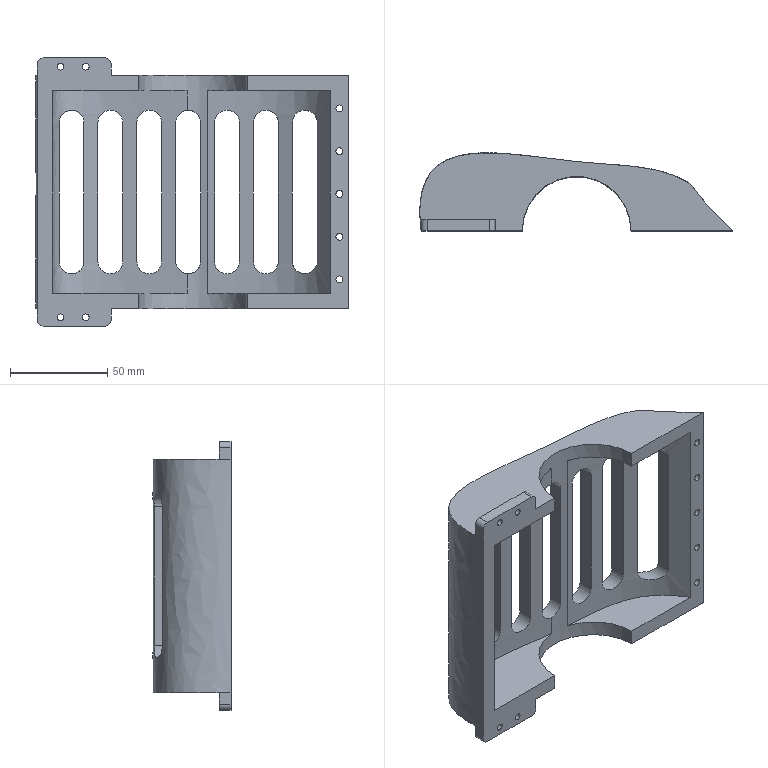Part | SolidWorks | features ICE 5, Fillet 2, Extrusion 1, MirrorPattern 1, Shell 1 | 1 solid | 80 faces | box 160.692 x 40.165 x 138 mm | volume 156504 mm3 | cylinder 45 | plane 32 | spline 3 | commonest cylinder face diameters 12.772 x21 3.6 x10 3.5 x8 6 x4 56 x1 360 x1